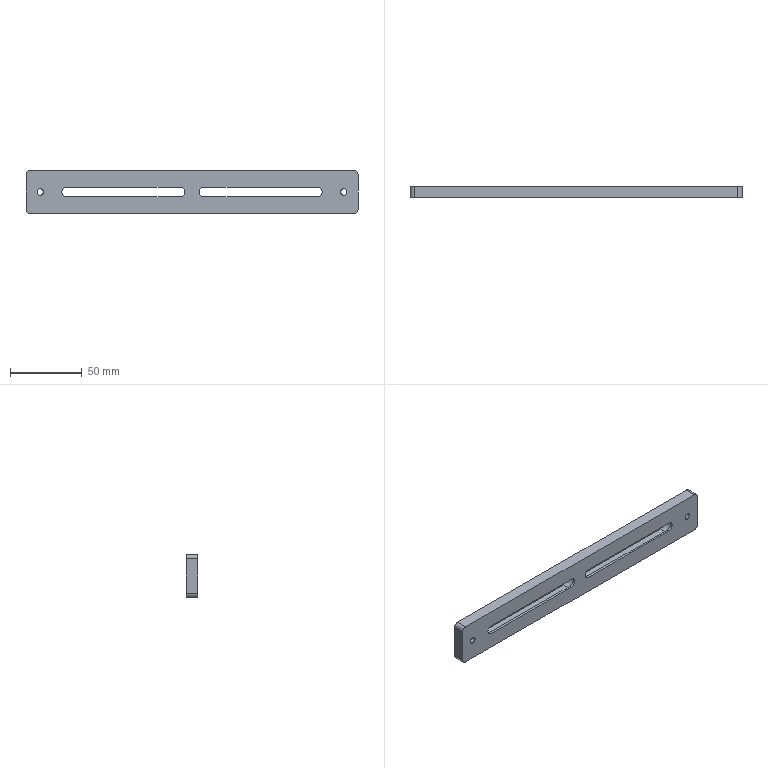Part | SolidWorks | features BaseBody 1 | 1 solid | 38 faces | box 232 x 8 x 30 mm | volume 40879 mm3 | cylinder 20 | plane 18 | commonest cylinder face diameters 4.5 x4 6 x4 6.6 x4 8 x4 11 x4
STEP:
#1=CARTESIAN_POINT('',(-106.,0.,-2.25));
#2=VERTEX_POINT('',#1);
#3=CARTESIAN_POINT('',(-106.,0.,2.25));
#4=VERTEX_POINT('',#3);
#5=CARTESIAN_POINT('',(-106.,0.,0.));
#6=DIRECTION('',(0.,1.,0.));
#7=DIRECTION('',(0.,0.,1.));
#8=AXIS2_PLACEMENT_3D('',#5,#6,#7);
#9=CIRCLE('',#8,2.25);
#10=EDGE_CURVE('',#2,#4,#9,.T.);
#11=ORIENTED_EDGE('',*,*,#10,.F.);
#12=CARTESIAN_POINT('',(-106.,3.6,-2.25));
#13=VERTEX_POINT('',#12);
#14=CARTESIAN_POINT('',(-106.,8.,-2.25));
#15=DIRECTION('',(0.,1.,0.));
#16=VECTOR('',#15,1000.);
#17=LINE('',#14,#16);
#18=EDGE_CURVE('',#2,#13,#17,.T.);
#19=ORIENTED_EDGE('',*,*,#18,.T.);
#20=CARTESIAN_POINT('',(-106.,3.6,2.25));
#21=VERTEX_POINT('',#20);
#22=CARTESIAN_POINT('',(-106.,3.6,0.));
#23=DIRECTION('',(0.,-1.,0.));
#24=DIRECTION('',(0.,0.,1.));
#25=AXIS2_PLACEMENT_3D('',#22,#23,#24);
#26=CIRCLE('',#25,2.25);
#27=EDGE_CURVE('',#21,#13,#26,.T.);
#28=ORIENTED_EDGE('',*,*,#27,.F.);
#29=CARTESIAN_POINT('',(-106.,8.,2.25));
#30=DIRECTION('',(0.,1.,0.));
#31=VECTOR('',#30,1000.);
#32=LINE('',#29,#31);
#33=EDGE_CURVE('',#4,#21,#32,.T.);
#34=ORIENTED_EDGE('',*,*,#33,.F.);
#35=EDGE_LOOP('',(#11,#19,#28,#34));
#36=FACE_OUTER_BOUND('',#35,.T.);
#37=CARTESIAN_POINT('',(-106.,8.,0.));
#38=DIRECTION('',(0.,1.,0.));
#39=DIRECTION('',(0.,0.,1.));
#40=AXIS2_PLACEMENT_3D('',#37,#38,#39);
#41=CYLINDRICAL_SURFACE('',#40,2.25);
#42=ADVANCED_FACE('',(#36),#41,.F.);
#43=CARTESIAN_POINT('',(106.,0.,-2.25));
#44=VERTEX_POINT('',#43);
#45=CARTESIAN_POINT('',(106.,0.,2.25));
#46=VERTEX_POINT('',#45);
#47=CARTESIAN_POINT('',(106.,0.,0.));
#48=DIRECTION('',(0.,1.,0.));
#49=DIRECTION('',(0.,0.,1.));
#50=AXIS2_PLACEMENT_3D('',#47,#48,#49);
#51=CIRCLE('',#50,2.25);
#52=EDGE_CURVE('',#44,#46,#51,.T.);
#53=ORIENTED_EDGE('',*,*,#52,.F.);
#54=CARTESIAN_POINT('',(106.,3.6,-2.25));
#55=VERTEX_POINT('',#54);
#56=CARTESIAN_POINT('',(106.,8.,-2.25));
#57=DIRECTION('',(0.,1.,0.));
#58=VECTOR('',#57,1000.);
#59=LINE('',#56,#58);
#60=EDGE_CURVE('',#44,#55,#59,.T.);
#61=ORIENTED_EDGE('',*,*,#60,.T.);
#62=CARTESIAN_POINT('',(106.,3.6,2.25));
#63=VERTEX_POINT('',#62);
#64=CARTESIAN_POINT('',(106.,3.6,0.));
#65=DIRECTION('',(0.,-1.,0.));
#66=DIRECTION('',(0.,0.,1.));
#67=AXIS2_PLACEMENT_3D('',#64,#65,#66);
#68=CIRCLE('',#67,2.25);
#69=EDGE_CURVE('',#63,#55,#68,.T.);
#70=ORIENTED_EDGE('',*,*,#69,.F.);
#71=CARTESIAN_POINT('',(106.,8.,2.25));
#72=DIRECTION('',(0.,1.,0.));
#73=VECTOR('',#72,1000.);
#74=LINE('',#71,#73);
#75=EDGE_CURVE('',#46,#63,#74,.T.);
#76=ORIENTED_EDGE('',*,*,#75,.F.);
#77=EDGE_LOOP('',(#53,#61,#70,#76));
#78=FACE_OUTER_BOUND('',#77,.T.);
#79=CARTESIAN_POINT('',(106.,8.,0.));
#80=DIRECTION('',(0.,1.,0.));
#81=DIRECTION('',(0.,0.,1.));
#82=AXIS2_PLACEMENT_3D('',#79,#80,#81);
#83=CYLINDRICAL_SURFACE('',#82,2.25);
#84=ADVANCED_FACE('',(#78),#83,.F.);
#85=CARTESIAN_POINT('',(-106.,3.6,4.));
#86=VERTEX_POINT('',#85);
#87=CARTESIAN_POINT('',(-106.,3.6,-4.));
#88=VERTEX_POINT('',#87);
#89=CARTESIAN_POINT('',(-106.,3.6,0.));
#90=DIRECTION('',(0.,-1.,0.));
#91=DIRECTION('',(0.,0.,1.));
#92=AXIS2_PLACEMENT_3D('',#89,#90,#91);
#93=CIRCLE('',#92,4.);
#94=EDGE_CURVE('',#86,#88,#93,.T.);
#95=ORIENTED_EDGE('',*,*,#94,.T.);
#96=CARTESIAN_POINT('',(-106.,8.,-4.));
#97=VERTEX_POINT('',#96);
#98=CARTESIAN_POINT('',(-106.,8.,-4.));
#99=DIRECTION('',(0.,1.,0.));
#100=VECTOR('',#99,1000.);
#101=LINE('',#98,#100);
#102=EDGE_CURVE('',#88,#97,#101,.T.);
#103=ORIENTED_EDGE('',*,*,#102,.T.);
#104=CARTESIAN_POINT('',(-106.,8.,4.));
#105=VERTEX_POINT('',#104);
#106=CARTESIAN_POINT('',(-106.,8.,0.));
#107=DIRECTION('',(0.,1.,0.));
#108=DIRECTION('',(0.,0.,1.));
#109=AXIS2_PLACEMENT_3D('',#106,#107,#108);
#110=CIRCLE('',#109,4.);
#111=EDGE_CURVE('',#97,#105,#110,.T.);
#112=ORIENTED_EDGE('',*,*,#111,.T.);
#113=CARTESIAN_POINT('',(-106.,8.,4.));
#114=DIRECTION('',(0.,1.,0.));
#115=VECTOR('',#114,1000.);
#116=LINE('',#113,#115);
#117=EDGE_CURVE('',#86,#105,#116,.T.);
#118=ORIENTED_EDGE('',*,*,#117,.F.);
#119=EDGE_LOOP('',(#95,#103,#112,#118));
#120=FACE_OUTER_BOUND('',#119,.T.);
#121=CARTESIAN_POINT('',(-106.,8.,0.));
#122=DIRECTION('',(0.,1.,0.));
#123=DIRECTION('',(0.,0.,1.));
#124=AXIS2_PLACEMENT_3D('',#121,#122,#123);
#125=CYLINDRICAL_SURFACE('',#124,4.);
#126=ADVANCED_FACE('',(#120),#125,.F.);
#127=CARTESIAN_POINT('',(106.,3.6,4.));
#128=VERTEX_POINT('',#127);
#129=CARTESIAN_POINT('',(106.,3.6,-4.));
#130=VERTEX_POINT('',#129);
#131=CARTESIAN_POINT('',(106.,3.6,0.));
#132=DIRECTION('',(0.,-1.,0.));
#133=DIRECTION('',(0.,0.,1.));
#134=AXIS2_PLACEMENT_3D('',#131,#132,#133);
#135=CIRCLE('',#134,4.);
#136=EDGE_CURVE('',#128,#130,#135,.T.);
#137=ORIENTED_EDGE('',*,*,#136,.T.);
#138=CARTESIAN_POINT('',(106.,8.,-4.));
#139=VERTEX_POINT('',#138);
#140=CARTESIAN_POINT('',(106.,8.,-4.));
#141=DIRECTION('',(0.,1.,0.));
#142=VECTOR('',#141,1000.);
#143=LINE('',#140,#142);
#144=EDGE_CURVE('',#130,#139,#143,.T.);
#145=ORIENTED_EDGE('',*,*,#144,.T.);
#146=CARTESIAN_POINT('',(106.,8.,4.));
#147=VERTEX_POINT('',#146);
#148=CARTESIAN_POINT('',(106.,8.,0.));
#149=DIRECTION('',(0.,1.,0.));
#150=DIRECTION('',(0.,0.,1.));
#151=AXIS2_PLACEMENT_3D('',#148,#149,#150);
#152=CIRCLE('',#151,4.);
#153=EDGE_CURVE('',#139,#147,#152,.T.);
#154=ORIENTED_EDGE('',*,*,#153,.T.);
#155=CARTESIAN_POINT('',(106.,8.,4.));
#156=DIRECTION('',(0.,1.,0.));
#157=VECTOR('',#156,1000.);
#158=LINE('',#155,#157);
#159=EDGE_CURVE('',#128,#147,#158,.T.);
#160=ORIENTED_EDGE('',*,*,#159,.F.);
#161=EDGE_LOOP('',(#137,#145,#154,#160));
#162=FACE_OUTER_BOUND('',#161,.T.);
#163=CARTESIAN_POINT('',(106.,8.,0.));
#164=DIRECTION('',(0.,1.,0.));
#165=DIRECTION('',(0.,0.,1.));
#166=AXIS2_PLACEMENT_3D('',#163,#164,#165);
#167=CYLINDRICAL_SURFACE('',#166,4.);
#168=ADVANCED_FACE('',(#162),#167,.F.);
#169=CARTESIAN_POINT('',(87.7,1.6,5.5));
#170=VERTEX_POINT('',#169);
#171=CARTESIAN_POINT('',(8.3,1.6,5.5));
#172=VERTEX_POINT('',#171);
#173=CARTESIAN_POINT('',(91.,1.6,5.5));
#174=DIRECTION('',(-1.,0.,0.));
#175=VECTOR('',#174,1000.);
#176=LINE('',#173,#175);
#177=EDGE_CURVE('',#170,#172,#176,.T.);
#178=ORIENTED_EDGE('',*,*,#177,.T.);
#179=CARTESIAN_POINT('',(8.3,8.,5.5));
#180=VERTEX_POINT('',#179);
#181=CARTESIAN_POINT('',(8.3,8.,5.5));
#182=DIRECTION('',(0.,1.,0.));
#183=VECTOR('',#182,1000.);
#184=LINE('',#181,#183);
#185=EDGE_CURVE('',#172,#180,#184,.T.);
#186=ORIENTED_EDGE('',*,*,#185,.T.);
#187=CARTESIAN_POINT('',(87.7,8.,5.5));
#188=VERTEX_POINT('',#187);
#189=CARTESIAN_POINT('',(0.,8.,5.5));
#190=DIRECTION('',(1.,0.,0.));
#191=VECTOR('',#190,1000.);
#192=LINE('',#189,#191);
#193=EDGE_CURVE('',#180,#188,#192,.T.);
#194=ORIENTED_EDGE('',*,*,#193,.T.);
#195=CARTESIAN_POINT('',(87.7,8.,5.5));
#196=DIRECTION('',(0.,-1.,0.));
#197=VECTOR('',#196,1000.);
#198=LINE('',#195,#197);
#199=EDGE_CURVE('',#188,#170,#198,.T.);
#200=ORIENTED_EDGE('',*,*,#199,.T.);
#201=EDGE_LOOP('',(#178,#186,#194,#200));
#202=FACE_OUTER_BOUND('',#201,.T.);
#203=CARTESIAN_POINT('',(8.3,8.,5.5));
#204=DIRECTION('',(0.,0.,1.));
#205=DIRECTION('',(1.,0.,0.));
#206=AXIS2_PLACEMENT_3D('',#203,#204,#205);
#207=PLANE('',#206);
#208=ADVANCED_FACE('',(#202),#207,.F.);
#209=ORIENTED_EDGE('',*,*,#185,.F.);
#210=CARTESIAN_POINT('',(8.3,1.6,-5.5));
#211=VERTEX_POINT('',#210);
#212=CARTESIAN_POINT('',(8.3,1.6,0.));
#213=DIRECTION('',(0.,-1.,0.));
#214=DIRECTION('',(0.,0.,1.));
#215=AXIS2_PLACEMENT_3D('',#212,#213,#214);
#216=CIRCLE('',#215,5.5);
#217=EDGE_CURVE('',#172,#211,#216,.T.);
#218=ORIENTED_EDGE('',*,*,#217,.T.);
#219=CARTESIAN_POINT('',(8.3,8.,-5.5));
#220=VERTEX_POINT('',#219);
#221=CARTESIAN_POINT('',(8.3,8.,-5.5));
#222=DIRECTION('',(0.,1.,0.));
#223=VECTOR('',#222,1000.);
#224=LINE('',#221,#223);
#225=EDGE_CURVE('',#211,#220,#224,.T.);
#226=ORIENTED_EDGE('',*,*,#225,.T.);
#227=CARTESIAN_POINT('',(8.3,8.,0.));
#228=DIRECTION('',(0.,1.,0.));
#229=DIRECTION('',(0.,0.,1.));
#230=AXIS2_PLACEMENT_3D('',#227,#228,#229);
#231=CIRCLE('',#230,5.5);
#232=EDGE_CURVE('',#220,#180,#231,.T.);
#233=ORIENTED_EDGE('',*,*,#232,.T.);
#234=EDGE_LOOP('',(#209,#218,#226,#233));
#235=FACE_OUTER_BOUND('',#234,.T.);
#236=CARTESIAN_POINT('',(8.3,8.,0.));
#237=DIRECTION('',(0.,1.,0.));
#238=DIRECTION('',(0.,0.,1.));
#239=AXIS2_PLACEMENT_3D('',#236,#237,#238);
#240=CYLINDRICAL_SURFACE('',#239,5.5);
#241=ADVANCED_FACE('',(#235),#240,.F.);
#242=CARTESIAN_POINT('',(87.7,8.,-5.5));
#243=VERTEX_POINT('',#242);
#244=CARTESIAN_POINT('',(0.,8.,-5.5));
#245=DIRECTION('',(-1.,0.,0.));
#246=VECTOR('',#245,1000.);
#247=LINE('',#244,#246);
#248=EDGE_CURVE('',#243,#220,#247,.T.);
#249=ORIENTED_EDGE('',*,*,#248,.T.);
#250=ORIENTED_EDGE('',*,*,#225,.F.);
#251=CARTESIAN_POINT('',(87.7,1.6,-5.5));
#252=VERTEX_POINT('',#251);
#253=CARTESIAN_POINT('',(91.,1.6,-5.5));
#254=DIRECTION('',(1.,0.,0.));
#255=VECTOR('',#254,1000.);
#256=LINE('',#253,#255);
#257=EDGE_CURVE('',#211,#252,#256,.T.);
#258=ORIENTED_EDGE('',*,*,#257,.T.);
#259=CARTESIAN_POINT('',(87.7,8.,-5.5));
#260=DIRECTION('',(0.,1.,0.));
#261=VECTOR('',#260,1000.);
#262=LINE('',#259,#261);
#263=EDGE_CURVE('',#252,#243,#262,.T.);
#264=ORIENTED_EDGE('',*,*,#263,.T.);
#265=EDGE_LOOP('',(#249,#250,#258,#264));
#266=FACE_OUTER_BOUND('',#265,.T.);
#267=CARTESIAN_POINT('',(8.3,8.,-5.5));
#268=DIRECTION('',(0.,0.,-1.));
#269=DIRECTION('',(-1.,0.,0.));
#270=AXIS2_PLACEMENT_3D('',#267,#268,#269);
#271=PLANE('',#270);
#272=ADVANCED_FACE('',(#266),#271,.F.);
#273=ORIENTED_EDGE('',*,*,#199,.F.);
#274=CARTESIAN_POINT('',(87.7,8.,0.));
#275=DIRECTION('',(0.,1.,0.));
#276=DIRECTION('',(0.,0.,1.));
#277=AXIS2_PLACEMENT_3D('',#274,#275,#276);
#278=CIRCLE('',#277,5.5);
#279=EDGE_CURVE('',#188,#243,#278,.T.);
#280=ORIENTED_EDGE('',*,*,#279,.T.);
#281=ORIENTED_EDGE('',*,*,#263,.F.);
#282=CARTESIAN_POINT('',(87.7,1.6,0.));
#283=DIRECTION('',(0.,-1.,0.));
#284=DIRECTION('',(0.,0.,1.));
#285=AXIS2_PLACEMENT_3D('',#282,#283,#284);
#286=CIRCLE('',#285,5.5);
#287=EDGE_CURVE('',#252,#170,#286,.T.);
#288=ORIENTED_EDGE('',*,*,#287,.T.);
#289=EDGE_LOOP('',(#273,#280,#281,#288));
#290=FACE_OUTER_BOUND('',#289,.T.);
#291=CARTESIAN_POINT('',(87.7,8.,0.));
#292=DIRECTION('',(0.,1.,0.));
#293=DIRECTION('',(0.,0.,1.));
#294=AXIS2_PLACEMENT_3D('',#291,#292,#293);
#295=CYLINDRICAL_SURFACE('',#294,5.5);
#296=ADVANCED_FACE('',(#290),#295,.F.);
#297=CARTESIAN_POINT('',(-8.3,1.6,5.5));
#298=VERTEX_POINT('',#297);
#299=CARTESIAN_POINT('',(-87.7,1.6,5.5));
#300=VERTEX_POINT('',#299);
#301=CARTESIAN_POINT('',(-5.,1.6,5.5));
#302=DIRECTION('',(-1.,0.,0.));
#303=VECTOR('',#302,1000.);
#304=LINE('',#301,#303);
#305=EDGE_CURVE('',#298,#300,#304,.T.);
#306=ORIENTED_EDGE('',*,*,#305,.T.);
#307=CARTESIAN_POINT('',(-87.7,8.,5.5));
#308=VERTEX_POINT('',#307);
#309=CARTESIAN_POINT('',(-87.7,8.,5.5));
#310=DIRECTION('',(0.,1.,0.));
#311=VECTOR('',#310,1000.);
#312=LINE('',#309,#311);
#313=EDGE_CURVE('',#300,#308,#312,.T.);
#314=ORIENTED_EDGE('',*,*,#313,.T.);
#315=CARTESIAN_POINT('',(-8.3,8.,5.5));
#316=VERTEX_POINT('',#315);
#317=CARTESIAN_POINT('',(0.,8.,5.5));
#318=DIRECTION('',(1.,0.,0.));
#319=VECTOR('',#318,1000.);
#320=LINE('',#317,#319);
#321=EDGE_CURVE('',#308,#316,#320,.T.);
#322=ORIENTED_EDGE('',*,*,#321,.T.);
#323=CARTESIAN_POINT('',(-8.3,8.,5.5));
#324=DIRECTION('',(0.,-1.,0.));
#325=VECTOR('',#324,1000.);
#326=LINE('',#323,#325);
#327=EDGE_CURVE('',#316,#298,#326,.T.);
#328=ORIENTED_EDGE('',*,*,#327,.T.);
#329=EDGE_LOOP('',(#306,#314,#322,#328));
#330=FACE_OUTER_BOUND('',#329,.T.);
#331=CARTESIAN_POINT('',(-87.7,8.,5.5));
#332=DIRECTION('',(0.,0.,1.));
#333=DIRECTION('',(1.,0.,0.));
#334=AXIS2_PLACEMENT_3D('',#331,#332,#333);
#335=PLANE('',#334);
#336=ADVANCED_FACE('',(#330),#335,.F.);
#337=ORIENTED_EDGE('',*,*,#313,.F.);
#338=CARTESIAN_POINT('',(-87.7,1.6,-5.5));
#339=VERTEX_POINT('',#338);
#340=CARTESIAN_POINT('',(-87.7,1.6,0.));
#341=DIRECTION('',(0.,-1.,0.));
#342=DIRECTION('',(0.,0.,1.));
#343=AXIS2_PLACEMENT_3D('',#340,#341,#342);
#344=CIRCLE('',#343,5.5);
#345=EDGE_CURVE('',#300,#339,#344,.T.);
#346=ORIENTED_EDGE('',*,*,#345,.T.);
#347=CARTESIAN_POINT('',(-87.7,8.,-5.5));
#348=VERTEX_POINT('',#347);
#349=CARTESIAN_POINT('',(-87.7,8.,-5.5));
#350=DIRECTION('',(0.,1.,0.));
#351=VECTOR('',#350,1000.);
#352=LINE('',#349,#351);
#353=EDGE_CURVE('',#339,#348,#352,.T.);
#354=ORIENTED_EDGE('',*,*,#353,.T.);
#355=CARTESIAN_POINT('',(-87.7,8.,0.));
#356=DIRECTION('',(0.,1.,0.));
#357=DIRECTION('',(0.,0.,1.));
#358=AXIS2_PLACEMENT_3D('',#355,#356,#357);
#359=CIRCLE('',#358,5.5);
#360=EDGE_CURVE('',#348,#308,#359,.T.);
#361=ORIENTED_EDGE('',*,*,#360,.T.);
#362=EDGE_LOOP('',(#337,#346,#354,#361));
#363=FACE_OUTER_BOUND('',#362,.T.);
#364=CARTESIAN_POINT('',(-87.7,8.,0.));
#365=DIRECTION('',(0.,1.,0.));
#366=DIRECTION('',(0.,0.,1.));
#367=AXIS2_PLACEMENT_3D('',#364,#365,#366);
#368=CYLINDRICAL_SURFACE('',#367,5.5);
#369=ADVANCED_FACE('',(#363),#368,.F.);
#370=CARTESIAN_POINT('',(-8.3,8.,-5.5));
#371=VERTEX_POINT('',#370);
#372=CARTESIAN_POINT('',(0.,8.,-5.5));
#373=DIRECTION('',(-1.,0.,0.));
#374=VECTOR('',#373,1000.);
#375=LINE('',#372,#374);
#376=EDGE_CURVE('',#371,#348,#375,.T.);
#377=ORIENTED_EDGE('',*,*,#376,.T.);
#378=ORIENTED_EDGE('',*,*,#353,.F.);
#379=CARTESIAN_POINT('',(-8.3,1.6,-5.5));
#380=VERTEX_POINT('',#379);
#381=CARTESIAN_POINT('',(-5.,1.6,-5.5));
#382=DIRECTION('',(1.,0.,0.));
#383=VECTOR('',#382,1000.);
#384=LINE('',#381,#383);
#385=EDGE_CURVE('',#339,#380,#384,.T.);
#386=ORIENTED_EDGE('',*,*,#385,.T.);
#387=CARTESIAN_POINT('',(-8.3,8.,-5.5));
#388=DIRECTION('',(0.,1.,0.));
#389=VECTOR('',#388,1000.);
#390=LINE('',#387,#389);
#391=EDGE_CURVE('',#380,#371,#390,.T.);
#392=ORIENTED_EDGE('',*,*,#391,.T.);
#393=EDGE_LOOP('',(#377,#378,#386,#392));
#394=FACE_OUTER_BOUND('',#393,.T.);
#395=CARTESIAN_POINT('',(-87.7,8.,-5.5));
#396=DIRECTION('',(0.,0.,-1.));
#397=DIRECTION('',(-1.,0.,0.));
#398=AXIS2_PLACEMENT_3D('',#395,#396,#397);
#399=PLANE('',#398);
#400=ADVANCED_FACE('',(#394),#399,.F.);
#401=ORIENTED_EDGE('',*,*,#327,.F.);
#402=CARTESIAN_POINT('',(-8.3,8.,0.));
#403=DIRECTION('',(0.,1.,0.));
#404=DIRECTION('',(0.,0.,1.));
#405=AXIS2_PLACEMENT_3D('',#402,#403,#404);
#406=CIRCLE('',#405,5.5);
#407=EDGE_CURVE('',#316,#371,#406,.T.);
#408=ORIENTED_EDGE('',*,*,#407,.T.);
#409=ORIENTED_EDGE('',*,*,#391,.F.);
#410=CARTESIAN_POINT('',(-8.3,1.6,0.));
#411=DIRECTION('',(0.,-1.,0.));
#412=DIRECTION('',(0.,0.,1.));
#413=AXIS2_PLACEMENT_3D('',#410,#411,#412);
#414=CIRCLE('',#413,5.5);
#415=EDGE_CURVE('',#380,#298,#414,.T.);
#416=ORIENTED_EDGE('',*,*,#415,.T.);
#417=EDGE_LOOP('',(#401,#408,#409,#416));
#418=FACE_OUTER_BOUND('',#417,.T.);
#419=CARTESIAN_POINT('',(-8.3,8.,0.));
#420=DIRECTION('',(0.,1.,0.));
#421=DIRECTION('',(0.,0.,1.));
#422=AXIS2_PLACEMENT_3D('',#419,#420,#421);
#423=CYLINDRICAL_SURFACE('',#422,5.5);
#424=ADVANCED_FACE('',(#418),#423,.F.);
#425=ORIENTED_EDGE('',*,*,#360,.F.);
#426=ORIENTED_EDGE('',*,*,#376,.F.);
#427=ORIENTED_EDGE('',*,*,#407,.F.);
#428=ORIENTED_EDGE('',*,*,#321,.F.);
#429=EDGE_LOOP('',(#425,#426,#427,#428));
#430=FACE_BOUND('',#429,.T.);
#431=ORIENTED_EDGE('',*,*,#248,.F.);
#432=ORIENTED_EDGE('',*,*,#279,.F.);
#433=ORIENTED_EDGE('',*,*,#193,.F.);
#434=ORIENTED_EDGE('',*,*,#232,.F.);
#435=EDGE_LOOP('',(#431,#432,#433,#434));
#436=FACE_BOUND('',#435,.T.);
#437=CARTESIAN_POINT('',(-106.,8.,0.));
#438=DIRECTION('',(0.,1.,0.));
#439=DIRECTION('',(0.,0.,1.));
#440=AXIS2_PLACEMENT_3D('',#437,#438,#439);
#441=CIRCLE('',#440,4.);
#442=EDGE_CURVE('',#105,#97,#441,.T.);
#443=ORIENTED_EDGE('',*,*,#442,.F.);
#444=ORIENTED_EDGE('',*,*,#111,.F.);
#445=EDGE_LOOP('',(#443,#444));
#446=FACE_BOUND('',#445,.T.);
#447=CARTESIAN_POINT('',(106.,8.,0.));
#448=DIRECTION('',(0.,1.,0.));
#449=DIRECTION('',(0.,0.,1.));
#450=AXIS2_PLACEMENT_3D('',#447,#448,#449);
#451=CIRCLE('',#450,4.);
#452=EDGE_CURVE('',#147,#139,#451,.T.);
#453=ORIENTED_EDGE('',*,*,#452,.F.);
#454=ORIENTED_EDGE('',*,*,#153,.F.);
#455=EDGE_LOOP('',(#453,#454));
#456=FACE_BOUND('',#455,.T.);
#457=CARTESIAN_POINT('',(-113.,8.,15.));
#458=VERTEX_POINT('',#457);
#459=CARTESIAN_POINT('',(-116.,8.,12.));
#460=VERTEX_POINT('',#459);
#461=CARTESIAN_POINT('',(-113.,8.,12.));
#462=DIRECTION('',(0.,-1.,0.));
#463=DIRECTION('',(0.,0.,-1.));
#464=AXIS2_PLACEMENT_3D('',#461,#462,#463);
#465=CIRCLE('',#464,3.);
#466=EDGE_CURVE('',#458,#460,#465,.T.);
#467=ORIENTED_EDGE('',*,*,#466,.F.);
#468=CARTESIAN_POINT('',(113.,8.,15.));
#469=VERTEX_POINT('',#468);
#470=CARTESIAN_POINT('',(-116.,8.,15.));
#471=DIRECTION('',(1.,0.,0.));
#472=VECTOR('',#471,1000.);
#473=LINE('',#470,#472);
#474=EDGE_CURVE('',#458,#469,#473,.T.);
#475=ORIENTED_EDGE('',*,*,#474,.T.);
#476=CARTESIAN_POINT('',(116.,8.,12.));
#477=VERTEX_POINT('',#476);
#478=CARTESIAN_POINT('',(113.,8.,12.));
#479=DIRECTION('',(0.,-1.,0.));
#480=DIRECTION('',(0.,0.,-1.));
#481=AXIS2_PLACEMENT_3D('',#478,#479,#480);
#482=CIRCLE('',#481,3.);
#483=EDGE_CURVE('',#477,#469,#482,.T.);
#484=ORIENTED_EDGE('',*,*,#483,.F.);
#485=CARTESIAN_POINT('',(116.,8.,-12.));
#486=VERTEX_POINT('',#485);
#487=CARTESIAN_POINT('',(116.,8.,15.));
#488=DIRECTION('',(0.,0.,-1.));
#489=VECTOR('',#488,1000.);
#490=LINE('',#487,#489);
#491=EDGE_CURVE('',#477,#486,#490,.T.);
#492=ORIENTED_EDGE('',*,*,#491,.T.);
#493=CARTESIAN_POINT('',(113.,8.,-15.));
#494=VERTEX_POINT('',#493);
#495=CARTESIAN_POINT('',(113.,8.,-12.));
#496=DIRECTION('',(0.,-1.,0.));
#497=DIRECTION('',(0.,0.,-1.));
#498=AXIS2_PLACEMENT_3D('',#495,#496,#497);
#499=CIRCLE('',#498,3.);
#500=EDGE_CURVE('',#494,#486,#499,.T.);
#501=ORIENTED_EDGE('',*,*,#500,.F.);
#502=CARTESIAN_POINT('',(-113.,8.,-15.));
#503=VERTEX_POINT('',#502);
#504=CARTESIAN_POINT('',(-116.,8.,-15.));
#505=DIRECTION('',(-1.,0.,0.));
#506=VECTOR('',#505,1000.);
#507=LINE('',#504,#506);
#508=EDGE_CURVE('',#494,#503,#507,.T.);
#509=ORIENTED_EDGE('',*,*,#508,.T.);
#510=CARTESIAN_POINT('',(-116.,8.,-12.));
#511=VERTEX_POINT('',#510);
#512=CARTESIAN_POINT('',(-113.,8.,-12.));
#513=DIRECTION('',(0.,-1.,0.));
#514=DIRECTION('',(0.,0.,-1.));
#515=AXIS2_PLACEMENT_3D('',#512,#513,#514);
#516=CIRCLE('',#515,3.);
#517=EDGE_CURVE('',#511,#503,#516,.T.);
#518=ORIENTED_EDGE('',*,*,#517,.F.);
#519=CARTESIAN_POINT('',(-116.,8.,15.));
#520=DIRECTION('',(0.,0.,1.));
#521=VECTOR('',#520,1000.);
#522=LINE('',#519,#521);
#523=EDGE_CURVE('',#511,#460,#522,.T.);
#524=ORIENTED_EDGE('',*,*,#523,.T.);
#525=EDGE_LOOP('',(#467,#475,#484,#492,#501,#509,#518,#524));
#526=FACE_OUTER_BOUND('',#525,.T.);
#527=CARTESIAN_POINT('',(0.,8.,0.));
#528=DIRECTION('',(0.,-1.,0.));
#529=DIRECTION('',(0.,0.,-1.));
#530=AXIS2_PLACEMENT_3D('',#527,#528,#529);
#531=PLANE('',#530);
#532=ADVANCED_FACE('',(#430,#436,#446,#456,#526),#531,.F.);
#533=ORIENTED_EDGE('',*,*,#69,.T.);
#534=CARTESIAN_POINT('',(106.,3.6,0.));
#535=DIRECTION('',(0.,-1.,0.));
#536=DIRECTION('',(0.,0.,1.));
#537=AXIS2_PLACEMENT_3D('',#534,#535,#536);
#538=CIRCLE('',#537,2.25);
#539=EDGE_CURVE('',#55,#63,#538,.T.);
#540=ORIENTED_EDGE('',*,*,#539,.T.);
#541=EDGE_LOOP('',(#533,#540));
#542=FACE_BOUND('',#541,.T.);
#543=ORIENTED_EDGE('',*,*,#136,.F.);
#544=CARTESIAN_POINT('',(106.,3.6,0.));
#545=DIRECTION('',(0.,-1.,0.));
#546=DIRECTION('',(0.,0.,1.));
#547=AXIS2_PLACEMENT_3D('',#544,#545,#546);
#548=CIRCLE('',#547,4.);
#549=EDGE_CURVE('',#130,#128,#548,.T.);
#550=ORIENTED_EDGE('',*,*,#549,.F.);
#551=EDGE_LOOP('',(#543,#550));
#552=FACE_OUTER_BOUND('',#551,.T.);
#553=CARTESIAN_POINT('',(108.25,3.6,0.));
#554=DIRECTION('',(0.,-1.,0.));
#555=DIRECTION('',(0.,0.,-1.));
#556=AXIS2_PLACEMENT_3D('',#553,#554,#555);
#557=PLANE('',#556);
#558=ADVANCED_FACE('',(#542,#552),#557,.F.);
#559=ORIENTED_EDGE('',*,*,#27,.T.);
#560=CARTESIAN_POINT('',(-106.,3.6,0.));
#561=DIRECTION('',(0.,-1.,0.));
#562=DIRECTION('',(0.,0.,1.));
#563=AXIS2_PLACEMENT_3D('',#560,#561,#562);
#564=CIRCLE('',#563,2.25);
#565=EDGE_CURVE('',#13,#21,#564,.T.);
#566=ORIENTED_EDGE('',*,*,#565,.T.);
#567=EDGE_LOOP('',(#559,#566));
#568=FACE_BOUND('',#567,.T.);
#569=ORIENTED_EDGE('',*,*,#94,.F.);
#570=CARTESIAN_POINT('',(-106.,3.6,0.));
#571=DIRECTION('',(0.,-1.,0.));
#572=DIRECTION('',(0.,0.,1.));
#573=AXIS2_PLACEMENT_3D('',#570,#571,#572);
#574=CIRCLE('',#573,4.);
#575=EDGE_CURVE('',#88,#86,#574,.T.);
#576=ORIENTED_EDGE('',*,*,#575,.F.);
#577=EDGE_LOOP('',(#569,#576));
#578=FACE_OUTER_BOUND('',#577,.T.);
#579=CARTESIAN_POINT('',(-103.75,3.6,0.));
#580=DIRECTION('',(0.,-1.,0.));
#581=DIRECTION('',(0.,0.,-1.));
#582=AXIS2_PLACEMENT_3D('',#579,#580,#581);
#583=PLANE('',#582);
#584=ADVANCED_FACE('',(#568,#578),#583,.F.);
#585=CARTESIAN_POINT('',(8.3,1.6,3.3));
#586=VERTEX_POINT('',#585);
#587=CARTESIAN_POINT('',(8.3,1.6,-3.3));
#588=VERTEX_POINT('',#587);
#589=CARTESIAN_POINT('',(8.3,1.6,0.));
#590=DIRECTION('',(0.,-1.,0.));
#591=DIRECTION('',(0.,0.,1.));
#592=AXIS2_PLACEMENT_3D('',#589,#590,#591);
#593=CIRCLE('',#592,3.3);
#594=EDGE_CURVE('',#586,#588,#593,.T.);
#595=ORIENTED_EDGE('',*,*,#594,.T.);
#596=CARTESIAN_POINT('',(87.7,1.6,-3.3));
#597=VERTEX_POINT('',#596);
#598=CARTESIAN_POINT('',(8.3,1.6,-3.3));
#599=DIRECTION('',(1.,0.,0.));
#600=VECTOR('',#599,1000.);
#601=LINE('',#598,#600);
#602=EDGE_CURVE('',#588,#597,#601,.T.);
#603=ORIENTED_EDGE('',*,*,#602,.T.);
#604=CARTESIAN_POINT('',(87.7,1.6,3.3));
#605=VERTEX_POINT('',#604);
#606=CARTESIAN_POINT('',(87.7,1.6,0.));
#607=DIRECTION('',(0.,-1.,0.));
#608=DIRECTION('',(0.,0.,1.));
#609=AXIS2_PLACEMENT_3D('',#606,#607,#608);
#610=CIRCLE('',#609,3.3);
#611=EDGE_CURVE('',#597,#605,#610,.T.);
#612=ORIENTED_EDGE('',*,*,#611,.T.);
#613=CARTESIAN_POINT('',(8.3,1.6,3.3));
#614=DIRECTION('',(-1.,0.,0.));
#615=VECTOR('',#614,1000.);
#616=LINE('',#613,#615);
#617=EDGE_CURVE('',#605,#586,#616,.T.);
#618=ORIENTED_EDGE('',*,*,#617,.T.);
#619=EDGE_LOOP('',(#595,#603,#612,#618));
#620=FACE_BOUND('',#619,.T.);
#621=ORIENTED_EDGE('',*,*,#257,.F.);
#622=ORIENTED_EDGE('',*,*,#217,.F.);
#623=ORIENTED_EDGE('',*,*,#177,.F.);
#624=ORIENTED_EDGE('',*,*,#287,.F.);
#625=EDGE_LOOP('',(#621,#622,#623,#624));
#626=FACE_OUTER_BOUND('',#625,.T.);
#627=CARTESIAN_POINT('',(91.,1.6,0.));
#628=DIRECTION('',(0.,-1.,0.));
#629=DIRECTION('',(0.,0.,-1.));
#630=AXIS2_PLACEMENT_3D('',#627,#628,#629);
#631=PLANE('',#630);
#632=ADVANCED_FACE('',(#620,#626),#631,.F.);
#633=CARTESIAN_POINT('',(-87.7,1.6,3.3));
#634=VERTEX_POINT('',#633);
#635=CARTESIAN_POINT('',(-87.7,1.6,-3.3));
#636=VERTEX_POINT('',#635);
#637=CARTESIAN_POINT('',(-87.7,1.6,0.));
#638=DIRECTION('',(0.,-1.,0.));
#639=DIRECTION('',(0.,0.,1.));
#640=AXIS2_PLACEMENT_3D('',#637,#638,#639);
#641=CIRCLE('',#640,3.3);
#642=EDGE_CURVE('',#634,#636,#641,.T.);
#643=ORIENTED_EDGE('',*,*,#642,.T.);
#644=CARTESIAN_POINT('',(-8.3,1.6,-3.3));
#645=VERTEX_POINT('',#644);
#646=CARTESIAN_POINT('',(-87.7,1.6,-3.3));
#647=DIRECTION('',(1.,0.,0.));
#648=VECTOR('',#647,1000.);
#649=LINE('',#646,#648);
#650=EDGE_CURVE('',#636,#645,#649,.T.);
#651=ORIENTED_EDGE('',*,*,#650,.T.);
#652=CARTESIAN_POINT('',(-8.3,1.6,3.3));
#653=VERTEX_POINT('',#652);
#654=CARTESIAN_POINT('',(-8.3,1.6,0.));
#655=DIRECTION('',(0.,-1.,0.));
#656=DIRECTION('',(0.,0.,1.));
#657=AXIS2_PLACEMENT_3D('',#654,#655,#656);
#658=CIRCLE('',#657,3.3);
#659=EDGE_CURVE('',#645,#653,#658,.T.);
#660=ORIENTED_EDGE('',*,*,#659,.T.);
#661=CARTESIAN_POINT('',(-87.7,1.6,3.3));
#662=DIRECTION('',(-1.,0.,0.));
#663=VECTOR('',#662,1000.);
#664=LINE('',#661,#663);
#665=EDGE_CURVE('',#653,#634,#664,.T.);
#666=ORIENTED_EDGE('',*,*,#665,.T.);
#667=EDGE_LOOP('',(#643,#651,#660,#666));
#668=FACE_BOUND('',#667,.T.);
#669=ORIENTED_EDGE('',*,*,#385,.F.);
#670=ORIENTED_EDGE('',*,*,#345,.F.);
#671=ORIENTED_EDGE('',*,*,#305,.F.);
#672=ORIENTED_EDGE('',*,*,#415,.F.);
#673=EDGE_LOOP('',(#669,#670,#671,#672));
#674=FACE_OUTER_BOUND('',#673,.T.);
#675=CARTESIAN_POINT('',(-5.,1.6,0.));
#676=DIRECTION('',(0.,-1.,0.));
#677=DIRECTION('',(0.,0.,-1.));
#678=AXIS2_PLACEMENT_3D('',#675,#676,#677);
#679=PLANE('',#678);
#680=ADVANCED_FACE('',(#668,#674),#679,.F.);
#681=CARTESIAN_POINT('',(-113.,0.,15.));
#682=VERTEX_POINT('',#681);
#683=CARTESIAN_POINT('',(-113.,8.,15.));
#684=DIRECTION('',(0.,1.,0.));
#685=VECTOR('',#684,1000.);
#686=LINE('',#683,#685);
#687=EDGE_CURVE('',#682,#458,#686,.T.);
#688=ORIENTED_EDGE('',*,*,#687,.F.);
#689=CARTESIAN_POINT('',(113.,0.,15.));
#690=VERTEX_POINT('',#689);
#691=CARTESIAN_POINT('',(0.,0.,15.));
#692=DIRECTION('',(-1.,0.,0.));
#693=VECTOR('',#692,1000.);
#694=LINE('',#691,#693);
#695=EDGE_CURVE('',#690,#682,#694,.T.);
#696=ORIENTED_EDGE('',*,*,#695,.F.);
#697=CARTESIAN_POINT('',(113.,8.,15.));
#698=DIRECTION('',(0.,-1.,0.));
#699=VECTOR('',#698,1000.);
#700=LINE('',#697,#699);
#701=EDGE_CURVE('',#469,#690,#700,.T.);
#702=ORIENTED_EDGE('',*,*,#701,.F.);
#703=ORIENTED_EDGE('',*,*,#474,.F.);
#704=EDGE_LOOP('',(#688,#696,#702,#703));
#705=FACE_OUTER_BOUND('',#704,.T.);
#706=CARTESIAN_POINT('',(-116.,8.,15.));
#707=DIRECTION('',(0.,0.,-1.));
#708=DIRECTION('',(0.,-1.,0.));
#709=AXIS2_PLACEMENT_3D('',#706,#707,#708);
#710=PLANE('',#709);
#711=ADVANCED_FACE('',(#705),#710,.F.);
#712=CARTESIAN_POINT('',(-116.,0.,12.));
#713=VERTEX_POINT('',#712);
#714=CARTESIAN_POINT('',(-113.,0.,12.));
#715=DIRECTION('',(0.,-1.,0.));
#716=DIRECTION('',(0.,0.,-1.));
#717=AXIS2_PLACEMENT_3D('',#714,#715,#716);
#718=CIRCLE('',#717,3.);
#719=EDGE_CURVE('',#682,#713,#718,.T.);
#720=ORIENTED_EDGE('',*,*,#719,.F.);
#721=ORIENTED_EDGE('',*,*,#687,.T.);
#722=ORIENTED_EDGE('',*,*,#466,.T.);
#723=CARTESIAN_POINT('',(-116.,8.,12.));
#724=DIRECTION('',(0.,-1.,0.));
#725=VECTOR('',#724,1000.);
#726=LINE('',#723,#725);
#727=EDGE_CURVE('',#460,#713,#726,.T.);
#728=ORIENTED_EDGE('',*,*,#727,.T.);
#729=EDGE_LOOP('',(#720,#721,#722,#728));
#730=FACE_OUTER_BOUND('',#729,.T.);
#731=CARTESIAN_POINT('',(-113.,8.,12.));
#732=DIRECTION('',(0.,-1.,0.));
#733=DIRECTION('',(0.,0.,-1.));
#734=AXIS2_PLACEMENT_3D('',#731,#732,#733);
#735=CYLINDRICAL_SURFACE('',#734,3.);
#736=ADVANCED_FACE('',(#730),#735,.T.);
#737=ORIENTED_EDGE('',*,*,#727,.F.);
#738=ORIENTED_EDGE('',*,*,#523,.F.);
#739=CARTESIAN_POINT('',(-116.,0.,-12.));
#740=VERTEX_POINT('',#739);
#741=CARTESIAN_POINT('',(-116.,8.,-12.));
#742=DIRECTION('',(0.,1.,0.));
#743=VECTOR('',#742,1000.);
#744=LINE('',#741,#743);
#745=EDGE_CURVE('',#740,#511,#744,.T.);
#746=ORIENTED_EDGE('',*,*,#745,.F.);
#747=CARTESIAN_POINT('',(-116.,0.,0.));
#748=DIRECTION('',(0.,0.,-1.));
#749=VECTOR('',#748,1000.);
#750=LINE('',#747,#749);
#751=EDGE_CURVE('',#713,#740,#750,.T.);
#752=ORIENTED_EDGE('',*,*,#751,.F.);
#753=EDGE_LOOP('',(#737,#738,#746,#752));
#754=FACE_OUTER_BOUND('',#753,.T.);
#755=CARTESIAN_POINT('',(-116.,8.,15.));
#756=DIRECTION('',(1.,0.,0.));
#757=DIRECTION('',(0.,1.,0.));
#758=AXIS2_PLACEMENT_3D('',#755,#756,#757);
#759=PLANE('',#758);
#760=ADVANCED_FACE('',(#754),#759,.F.);
#761=CARTESIAN_POINT('',(-113.,0.,-15.));
#762=VERTEX_POINT('',#761);
#763=CARTESIAN_POINT('',(-113.,0.,-12.));
#764=DIRECTION('',(0.,-1.,0.));
#765=DIRECTION('',(0.,0.,-1.));
#766=AXIS2_PLACEMENT_3D('',#763,#764,#765);
#767=CIRCLE('',#766,3.);
#768=EDGE_CURVE('',#740,#762,#767,.T.);
#769=ORIENTED_EDGE('',*,*,#768,.F.);
#770=ORIENTED_EDGE('',*,*,#745,.T.);
#771=ORIENTED_EDGE('',*,*,#517,.T.);
#772=CARTESIAN_POINT('',(-113.,8.,-15.));
#773=DIRECTION('',(0.,-1.,0.));
#774=VECTOR('',#773,1000.);
#775=LINE('',#772,#774);
#776=EDGE_CURVE('',#503,#762,#775,.T.);
#777=ORIENTED_EDGE('',*,*,#776,.T.);
#778=EDGE_LOOP('',(#769,#770,#771,#777));
#779=FACE_OUTER_BOUND('',#778,.T.);
#780=CARTESIAN_POINT('',(-113.,8.,-12.));
#781=DIRECTION('',(0.,-1.,0.));
#782=DIRECTION('',(0.,0.,-1.));
#783=AXIS2_PLACEMENT_3D('',#780,#781,#782);
#784=CYLINDRICAL_SURFACE('',#783,3.);
#785=ADVANCED_FACE('',(#779),#784,.T.);
#786=ORIENTED_EDGE('',*,*,#776,.F.);
#787=ORIENTED_EDGE('',*,*,#508,.F.);
#788=CARTESIAN_POINT('',(113.,0.,-15.));
#789=VERTEX_POINT('',#788);
#790=CARTESIAN_POINT('',(113.,8.,-15.));
#791=DIRECTION('',(0.,1.,0.));
#792=VECTOR('',#791,1000.);
#793=LINE('',#790,#792);
#794=EDGE_CURVE('',#789,#494,#793,.T.);
#795=ORIENTED_EDGE('',*,*,#794,.F.);
#796=CARTESIAN_POINT('',(0.,0.,-15.));
#797=DIRECTION('',(1.,0.,0.));
#798=VECTOR('',#797,1000.);
#799=LINE('',#796,#798);
#800=EDGE_CURVE('',#762,#789,#799,.T.);
#801=ORIENTED_EDGE('',*,*,#800,.F.);
#802=EDGE_LOOP('',(#786,#787,#795,#801));
#803=FACE_OUTER_BOUND('',#802,.T.);
#804=CARTESIAN_POINT('',(-116.,8.,-15.));
#805=DIRECTION('',(0.,0.,1.));
#806=DIRECTION('',(1.,0.,0.));
#807=AXIS2_PLACEMENT_3D('',#804,#805,#806);
#808=PLANE('',#807);
#809=ADVANCED_FACE('',(#803),#808,.F.);
#810=CARTESIAN_POINT('',(116.,0.,-12.));
#811=VERTEX_POINT('',#810);
#812=CARTESIAN_POINT('',(113.,0.,-12.));
#813=DIRECTION('',(0.,-1.,0.));
#814=DIRECTION('',(0.,0.,-1.));
#815=AXIS2_PLACEMENT_3D('',#812,#813,#814);
#816=CIRCLE('',#815,3.);
#817=EDGE_CURVE('',#789,#811,#816,.T.);
#818=ORIENTED_EDGE('',*,*,#817,.F.);
#819=ORIENTED_EDGE('',*,*,#794,.T.);
#820=ORIENTED_EDGE('',*,*,#500,.T.);
#821=CARTESIAN_POINT('',(116.,8.,-12.));
#822=DIRECTION('',(0.,-1.,0.));
#823=VECTOR('',#822,1000.);
#824=LINE('',#821,#823);
#825=EDGE_CURVE('',#486,#811,#824,.T.);
#826=ORIENTED_EDGE('',*,*,#825,.T.);
#827=EDGE_LOOP('',(#818,#819,#820,#826));
#828=FACE_OUTER_BOUND('',#827,.T.);
#829=CARTESIAN_POINT('',(113.,8.,-12.));
#830=DIRECTION('',(0.,-1.,0.));
#831=DIRECTION('',(0.,0.,-1.));
#832=AXIS2_PLACEMENT_3D('',#829,#830,#831);
#833=CYLINDRICAL_SURFACE('',#832,3.);
#834=ADVANCED_FACE('',(#828),#833,.T.);
#835=CARTESIAN_POINT('',(116.,0.,12.));
#836=VERTEX_POINT('',#835);
#837=CARTESIAN_POINT('',(116.,8.,12.));
#838=DIRECTION('',(0.,1.,0.));
#839=VECTOR('',#838,1000.);
#840=LINE('',#837,#839);
#841=EDGE_CURVE('',#836,#477,#840,.T.);
#842=ORIENTED_EDGE('',*,*,#841,.F.);
#843=CARTESIAN_POINT('',(116.,0.,0.));
#844=DIRECTION('',(0.,0.,1.));
#845=VECTOR('',#844,1000.);
#846=LINE('',#843,#845);
#847=EDGE_CURVE('',#811,#836,#846,.T.);
#848=ORIENTED_EDGE('',*,*,#847,.F.);
#849=ORIENTED_EDGE('',*,*,#825,.F.);
#850=ORIENTED_EDGE('',*,*,#491,.F.);
#851=EDGE_LOOP('',(#842,#848,#849,#850));
#852=FACE_OUTER_BOUND('',#851,.T.);
#853=CARTESIAN_POINT('',(116.,8.,15.));
#854=DIRECTION('',(-1.,0.,0.));
#855=DIRECTION('',(0.,0.,1.));
#856=AXIS2_PLACEMENT_3D('',#853,#854,#855);
#857=PLANE('',#856);
#858=ADVANCED_FACE('',(#852),#857,.F.);
#859=CARTESIAN_POINT('',(113.,0.,12.));
#860=DIRECTION('',(0.,-1.,0.));
#861=DIRECTION('',(0.,0.,-1.));
#862=AXIS2_PLACEMENT_3D('',#859,#860,#861);
#863=CIRCLE('',#862,3.);
#864=EDGE_CURVE('',#836,#690,#863,.T.);
#865=ORIENTED_EDGE('',*,*,#864,.F.);
#866=ORIENTED_EDGE('',*,*,#841,.T.);
#867=ORIENTED_EDGE('',*,*,#483,.T.);
#868=ORIENTED_EDGE('',*,*,#701,.T.);
#869=EDGE_LOOP('',(#865,#866,#867,#868));
#870=FACE_OUTER_BOUND('',#869,.T.);
#871=CARTESIAN_POINT('',(113.,8.,12.));
#872=DIRECTION('',(0.,-1.,0.));
#873=DIRECTION('',(0.,0.,-1.));
#874=AXIS2_PLACEMENT_3D('',#871,#872,#873);
#875=CYLINDRICAL_SURFACE('',#874,3.);
#876=ADVANCED_FACE('',(#870),#875,.T.);
#877=ORIENTED_EDGE('',*,*,#602,.F.);
#878=CARTESIAN_POINT('',(8.3,0.,-3.3));
#879=VERTEX_POINT('',#878);
#880=CARTESIAN_POINT('',(8.3,8.,-3.3));
#881=DIRECTION('',(0.,-1.,0.));
#882=VECTOR('',#881,1000.);
#883=LINE('',#880,#882);
#884=EDGE_CURVE('',#588,#879,#883,.T.);
#885=ORIENTED_EDGE('',*,*,#884,.T.);
#886=CARTESIAN_POINT('',(87.7,0.,-3.3));
#887=VERTEX_POINT('',#886);
#888=CARTESIAN_POINT('',(0.,0.,-3.3));
#889=DIRECTION('',(-1.,0.,0.));
#890=VECTOR('',#889,1000.);
#891=LINE('',#888,#890);
#892=EDGE_CURVE('',#887,#879,#891,.T.);
#893=ORIENTED_EDGE('',*,*,#892,.F.);
#894=CARTESIAN_POINT('',(87.7,8.,-3.3));
#895=DIRECTION('',(0.,1.,0.));
#896=VECTOR('',#895,1000.);
#897=LINE('',#894,#896);
#898=EDGE_CURVE('',#887,#597,#897,.T.);
#899=ORIENTED_EDGE('',*,*,#898,.T.);
#900=EDGE_LOOP('',(#877,#885,#893,#899));
#901=FACE_OUTER_BOUND('',#900,.T.);
#902=CARTESIAN_POINT('',(8.3,8.,-3.3));
#903=DIRECTION('',(0.,0.,-1.));
#904=DIRECTION('',(-1.,0.,0.));
#905=AXIS2_PLACEMENT_3D('',#902,#903,#904);
#906=PLANE('',#905);
#907=ADVANCED_FACE('',(#901),#906,.F.);
#908=CARTESIAN_POINT('',(8.3,0.,3.3));
#909=VERTEX_POINT('',#908);
#910=CARTESIAN_POINT('',(8.3,8.,3.3));
#911=DIRECTION('',(0.,-1.,0.));
#912=VECTOR('',#911,1000.);
#913=LINE('',#910,#912);
#914=EDGE_CURVE('',#586,#909,#913,.T.);
#915=ORIENTED_EDGE('',*,*,#914,.T.);
#916=CARTESIAN_POINT('',(8.3,0.,0.));
#917=DIRECTION('',(0.,1.,0.));
#918=DIRECTION('',(0.,0.,1.));
#919=AXIS2_PLACEMENT_3D('',#916,#917,#918);
#920=CIRCLE('',#919,3.3);
#921=EDGE_CURVE('',#879,#909,#920,.T.);
#922=ORIENTED_EDGE('',*,*,#921,.F.);
#923=ORIENTED_EDGE('',*,*,#884,.F.);
#924=ORIENTED_EDGE('',*,*,#594,.F.);
#925=EDGE_LOOP('',(#915,#922,#923,#924));
#926=FACE_OUTER_BOUND('',#925,.T.);
#927=CARTESIAN_POINT('',(8.3,8.,0.));
#928=DIRECTION('',(0.,1.,0.));
#929=DIRECTION('',(0.,0.,1.));
#930=AXIS2_PLACEMENT_3D('',#927,#928,#929);
#931=CYLINDRICAL_SURFACE('',#930,3.3);
#932=ADVANCED_FACE('',(#926),#931,.F.);
#933=CARTESIAN_POINT('',(87.7,0.,3.3));
#934=VERTEX_POINT('',#933);
#935=CARTESIAN_POINT('',(0.,0.,3.3));
#936=DIRECTION('',(1.,0.,0.));
#937=VECTOR('',#936,1000.);
#938=LINE('',#935,#937);
#939=EDGE_CURVE('',#909,#934,#938,.T.);
#940=ORIENTED_EDGE('',*,*,#939,.F.);
#941=ORIENTED_EDGE('',*,*,#914,.F.);
#942=ORIENTED_EDGE('',*,*,#617,.F.);
#943=CARTESIAN_POINT('',(87.7,8.,3.3));
#944=DIRECTION('',(0.,-1.,0.));
#945=VECTOR('',#944,1000.);
#946=LINE('',#943,#945);
#947=EDGE_CURVE('',#605,#934,#946,.T.);
#948=ORIENTED_EDGE('',*,*,#947,.T.);
#949=EDGE_LOOP('',(#940,#941,#942,#948));
#950=FACE_OUTER_BOUND('',#949,.T.);
#951=CARTESIAN_POINT('',(8.3,8.,3.3));
#952=DIRECTION('',(0.,0.,1.));
#953=DIRECTION('',(1.,0.,0.));
#954=AXIS2_PLACEMENT_3D('',#951,#952,#953);
#955=PLANE('',#954);
#956=ADVANCED_FACE('',(#950),#955,.F.);
#957=ORIENTED_EDGE('',*,*,#947,.F.);
#958=ORIENTED_EDGE('',*,*,#611,.F.);
#959=ORIENTED_EDGE('',*,*,#898,.F.);
#960=CARTESIAN_POINT('',(87.7,0.,0.));
#961=DIRECTION('',(0.,1.,0.));
#962=DIRECTION('',(0.,0.,1.));
#963=AXIS2_PLACEMENT_3D('',#960,#961,#962);
#964=CIRCLE('',#963,3.3);
#965=EDGE_CURVE('',#934,#887,#964,.T.);
#966=ORIENTED_EDGE('',*,*,#965,.F.);
#967=EDGE_LOOP('',(#957,#958,#959,#966));
#968=FACE_OUTER_BOUND('',#967,.T.);
#969=CARTESIAN_POINT('',(87.7,8.,0.));
#970=DIRECTION('',(0.,1.,0.));
#971=DIRECTION('',(0.,0.,1.));
#972=AXIS2_PLACEMENT_3D('',#969,#970,#971);
#973=CYLINDRICAL_SURFACE('',#972,3.3);
#974=ADVANCED_FACE('',(#968),#973,.F.);
#975=ORIENTED_EDGE('',*,*,#650,.F.);
#976=CARTESIAN_POINT('',(-87.7,0.,-3.3));
#977=VERTEX_POINT('',#976);
#978=CARTESIAN_POINT('',(-87.7,8.,-3.3));
#979=DIRECTION('',(0.,-1.,0.));
#980=VECTOR('',#979,1000.);
#981=LINE('',#978,#980);
#982=EDGE_CURVE('',#636,#977,#981,.T.);
#983=ORIENTED_EDGE('',*,*,#982,.T.);
#984=CARTESIAN_POINT('',(-8.3,0.,-3.3));
#985=VERTEX_POINT('',#984);
#986=CARTESIAN_POINT('',(0.,0.,-3.3));
#987=DIRECTION('',(-1.,0.,0.));
#988=VECTOR('',#987,1000.);
#989=LINE('',#986,#988);
#990=EDGE_CURVE('',#985,#977,#989,.T.);
#991=ORIENTED_EDGE('',*,*,#990,.F.);
#992=CARTESIAN_POINT('',(-8.3,8.,-3.3));
#993=DIRECTION('',(0.,1.,0.));
#994=VECTOR('',#993,1000.);
#995=LINE('',#992,#994);
#996=EDGE_CURVE('',#985,#645,#995,.T.);
#997=ORIENTED_EDGE('',*,*,#996,.T.);
#998=EDGE_LOOP('',(#975,#983,#991,#997));
#999=FACE_OUTER_BOUND('',#998,.T.);
#1000=CARTESIAN_POINT('',(-87.7,8.,-3.3));
#1001=DIRECTION('',(0.,0.,-1.));
#1002=DIRECTION('',(-1.,0.,0.));
#1003=AXIS2_PLACEMENT_3D('',#1000,#1001,#1002);
#1004=PLANE('',#1003);
#1005=ADVANCED_FACE('',(#999),#1004,.F.);
#1006=CARTESIAN_POINT('',(-87.7,0.,3.3));
#1007=VERTEX_POINT('',#1006);
#1008=CARTESIAN_POINT('',(-87.7,8.,3.3));
#1009=DIRECTION('',(0.,-1.,0.));
#1010=VECTOR('',#1009,1000.);
#1011=LINE('',#1008,#1010);
#1012=EDGE_CURVE('',#634,#1007,#1011,.T.);
#1013=ORIENTED_EDGE('',*,*,#1012,.T.);
#1014=CARTESIAN_POINT('',(-87.7,0.,0.));
#1015=DIRECTION('',(0.,1.,0.));
#1016=DIRECTION('',(0.,0.,1.));
#1017=AXIS2_PLACEMENT_3D('',#1014,#1015,#1016);
#1018=CIRCLE('',#1017,3.3);
#1019=EDGE_CURVE('',#977,#1007,#1018,.T.);
#1020=ORIENTED_EDGE('',*,*,#1019,.F.);
#1021=ORIENTED_EDGE('',*,*,#982,.F.);
#1022=ORIENTED_EDGE('',*,*,#642,.F.);
#1023=EDGE_LOOP('',(#1013,#1020,#1021,#1022));
#1024=FACE_OUTER_BOUND('',#1023,.T.);
#1025=CARTESIAN_POINT('',(-87.7,8.,0.));
#1026=DIRECTION('',(0.,1.,0.));
#1027=DIRECTION('',(0.,0.,1.));
#1028=AXIS2_PLACEMENT_3D('',#1025,#1026,#1027);
#1029=CYLINDRICAL_SURFACE('',#1028,3.3);
#1030=ADVANCED_FACE('',(#1024),#1029,.F.);
#1031=CARTESIAN_POINT('',(-8.3,0.,3.3));
#1032=VERTEX_POINT('',#1031);
#1033=CARTESIAN_POINT('',(0.,0.,3.3));
#1034=DIRECTION('',(1.,0.,0.));
#1035=VECTOR('',#1034,1000.);
#1036=LINE('',#1033,#1035);
#1037=EDGE_CURVE('',#1007,#1032,#1036,.T.);
#1038=ORIENTED_EDGE('',*,*,#1037,.F.);
#1039=ORIENTED_EDGE('',*,*,#1012,.F.);
#1040=ORIENTED_EDGE('',*,*,#665,.F.);
#1041=CARTESIAN_POINT('',(-8.3,8.,3.3));
#1042=DIRECTION('',(0.,-1.,0.));
#1043=VECTOR('',#1042,1000.);
#1044=LINE('',#1041,#1043);
#1045=EDGE_CURVE('',#653,#1032,#1044,.T.);
#1046=ORIENTED_EDGE('',*,*,#1045,.T.);
#1047=EDGE_LOOP('',(#1038,#1039,#1040,#1046));
#1048=FACE_OUTER_BOUND('',#1047,.T.);
#1049=CARTESIAN_POINT('',(-87.7,8.,3.3));
#1050=DIRECTION('',(0.,0.,1.));
#1051=DIRECTION('',(1.,0.,0.));
#1052=AXIS2_PLACEMENT_3D('',#1049,#1050,#1051);
#1053=PLANE('',#1052);
#1054=ADVANCED_FACE('',(#1048),#1053,.F.);
#1055=ORIENTED_EDGE('',*,*,#1045,.F.);
#1056=ORIENTED_EDGE('',*,*,#659,.F.);
#1057=ORIENTED_EDGE('',*,*,#996,.F.);
#1058=CARTESIAN_POINT('',(-8.3,0.,0.));
#1059=DIRECTION('',(0.,1.,0.));
#1060=DIRECTION('',(0.,0.,1.));
#1061=AXIS2_PLACEMENT_3D('',#1058,#1059,#1060);
#1062=CIRCLE('',#1061,3.3);
#1063=EDGE_CURVE('',#1032,#985,#1062,.T.);
#1064=ORIENTED_EDGE('',*,*,#1063,.F.);
#1065=EDGE_LOOP('',(#1055,#1056,#1057,#1064));
#1066=FACE_OUTER_BOUND('',#1065,.T.);
#1067=CARTESIAN_POINT('',(-8.3,8.,0.));
#1068=DIRECTION('',(0.,1.,0.));
#1069=DIRECTION('',(0.,0.,1.));
#1070=AXIS2_PLACEMENT_3D('',#1067,#1068,#1069);
#1071=CYLINDRICAL_SURFACE('',#1070,3.3);
#1072=ADVANCED_FACE('',(#1066),#1071,.F.);
#1073=CARTESIAN_POINT('',(106.,0.,0.));
#1074=DIRECTION('',(0.,1.,0.));
#1075=DIRECTION('',(0.,0.,1.));
#1076=AXIS2_PLACEMENT_3D('',#1073,#1074,#1075);
#1077=CIRCLE('',#1076,2.25);
#1078=EDGE_CURVE('',#46,#44,#1077,.T.);
#1079=ORIENTED_EDGE('',*,*,#1078,.T.);
#1080=ORIENTED_EDGE('',*,*,#52,.T.);
#1081=EDGE_LOOP('',(#1079,#1080));
#1082=FACE_BOUND('',#1081,.T.);
#1083=CARTESIAN_POINT('',(-106.,0.,0.));
#1084=DIRECTION('',(0.,1.,0.));
#1085=DIRECTION('',(0.,0.,1.));
#1086=AXIS2_PLACEMENT_3D('',#1083,#1084,#1085);
#1087=CIRCLE('',#1086,2.25);
#1088=EDGE_CURVE('',#4,#2,#1087,.T.);
#1089=ORIENTED_EDGE('',*,*,#1088,.T.);
#1090=ORIENTED_EDGE('',*,*,#10,.T.);
#1091=EDGE_LOOP('',(#1089,#1090));
#1092=FACE_BOUND('',#1091,.T.);
#1093=ORIENTED_EDGE('',*,*,#939,.T.);
#1094=ORIENTED_EDGE('',*,*,#965,.T.);
#1095=ORIENTED_EDGE('',*,*,#892,.T.);
#1096=ORIENTED_EDGE('',*,*,#921,.T.);
#1097=EDGE_LOOP('',(#1093,#1094,#1095,#1096));
#1098=FACE_BOUND('',#1097,.T.);
#1099=ORIENTED_EDGE('',*,*,#1037,.T.);
#1100=ORIENTED_EDGE('',*,*,#1063,.T.);
#1101=ORIENTED_EDGE('',*,*,#990,.T.);
#1102=ORIENTED_EDGE('',*,*,#1019,.T.);
#1103=EDGE_LOOP('',(#1099,#1100,#1101,#1102));
#1104=FACE_BOUND('',#1103,.T.);
#1105=ORIENTED_EDGE('',*,*,#847,.T.);
#1106=ORIENTED_EDGE('',*,*,#864,.T.);
#1107=ORIENTED_EDGE('',*,*,#695,.T.);
#1108=ORIENTED_EDGE('',*,*,#719,.T.);
#1109=ORIENTED_EDGE('',*,*,#751,.T.);
#1110=ORIENTED_EDGE('',*,*,#768,.T.);
#1111=ORIENTED_EDGE('',*,*,#800,.T.);
#1112=ORIENTED_EDGE('',*,*,#817,.T.);
#1113=EDGE_LOOP('',(#1105,#1106,#1107,#1108,#1109,#1110,#1111,#1112));
#1114=FACE_OUTER_BOUND('',#1113,.T.);
#1115=CARTESIAN_POINT('',(0.,0.,0.));
#1116=DIRECTION('',(0.,-1.,0.));
#1117=DIRECTION('',(0.,0.,-1.));
#1118=AXIS2_PLACEMENT_3D('',#1115,#1116,#1117);
#1119=PLANE('',#1118);
#1120=ADVANCED_FACE('',(#1082,#1092,#1098,#1104,#1114),#1119,.T.);
#1121=ORIENTED_EDGE('',*,*,#144,.F.);
#1122=ORIENTED_EDGE('',*,*,#549,.T.);
#1123=ORIENTED_EDGE('',*,*,#159,.T.);
#1124=ORIENTED_EDGE('',*,*,#452,.T.);
#1125=EDGE_LOOP('',(#1121,#1122,#1123,#1124));
#1126=FACE_OUTER_BOUND('',#1125,.T.);
#1127=CARTESIAN_POINT('',(106.,8.,0.));
#1128=DIRECTION('',(0.,1.,0.));
#1129=DIRECTION('',(0.,0.,1.));
#1130=AXIS2_PLACEMENT_3D('',#1127,#1128,#1129);
#1131=CYLINDRICAL_SURFACE('',#1130,4.);
#1132=ADVANCED_FACE('',(#1126),#1131,.F.);
#1133=ORIENTED_EDGE('',*,*,#102,.F.);
#1134=ORIENTED_EDGE('',*,*,#575,.T.);
#1135=ORIENTED_EDGE('',*,*,#117,.T.);
#1136=ORIENTED_EDGE('',*,*,#442,.T.);
#1137=EDGE_LOOP('',(#1133,#1134,#1135,#1136));
#1138=FACE_OUTER_BOUND('',#1137,.T.);
#1139=CARTESIAN_POINT('',(-106.,8.,0.));
#1140=DIRECTION('',(0.,1.,0.));
#1141=DIRECTION('',(0.,0.,1.));
#1142=AXIS2_PLACEMENT_3D('',#1139,#1140,#1141);
#1143=CYLINDRICAL_SURFACE('',#1142,4.);
#1144=ADVANCED_FACE('',(#1138),#1143,.F.);
#1145=ORIENTED_EDGE('',*,*,#60,.F.);
#1146=ORIENTED_EDGE('',*,*,#1078,.F.);
#1147=ORIENTED_EDGE('',*,*,#75,.T.);
#1148=ORIENTED_EDGE('',*,*,#539,.F.);
#1149=EDGE_LOOP('',(#1145,#1146,#1147,#1148));
#1150=FACE_OUTER_BOUND('',#1149,.T.);
#1151=CARTESIAN_POINT('',(106.,8.,0.));
#1152=DIRECTION('',(0.,1.,0.));
#1153=DIRECTION('',(0.,0.,1.));
#1154=AXIS2_PLACEMENT_3D('',#1151,#1152,#1153);
#1155=CYLINDRICAL_SURFACE('',#1154,2.25);
#1156=ADVANCED_FACE('',(#1150),#1155,.F.);
#1157=ORIENTED_EDGE('',*,*,#18,.F.);
#1158=ORIENTED_EDGE('',*,*,#1088,.F.);
#1159=ORIENTED_EDGE('',*,*,#33,.T.);
#1160=ORIENTED_EDGE('',*,*,#565,.F.);
#1161=EDGE_LOOP('',(#1157,#1158,#1159,#1160));
#1162=FACE_OUTER_BOUND('',#1161,.T.);
#1163=CARTESIAN_POINT('',(-106.,8.,0.));
#1164=DIRECTION('',(0.,1.,0.));
#1165=DIRECTION('',(0.,0.,1.));
#1166=AXIS2_PLACEMENT_3D('',#1163,#1164,#1165);
#1167=CYLINDRICAL_SURFACE('',#1166,2.25);
#1168=ADVANCED_FACE('',(#1162),#1167,.F.);
#1169=CLOSED_SHELL('',(#42,#84,#126,#168,#208,#241,#272,#296,#336,#369,#400,#424,#532,#558,#584,#632,#680,#711,#736,#760,#785,#809,#834,#858,#876,#907,#932,#956,#974,#1005,#1030,#1054,#1072,#1120,#1132,#1144,#1156,#1168));
#1170=MANIFOLD_SOLID_BREP('',#1169);
#1171=CARTESIAN_POINT('',(0.,0.,0.));
#1172=DIRECTION('',(0.,0.,1.));
#1173=DIRECTION('',(1.,0.,0.));
#1174=AXIS2_PLACEMENT_3D('',#1171,#1172,#1173);
#1175=(LENGTH_UNIT()NAMED_UNIT(*)SI_UNIT(.MILLI.,.METRE.));
#1176=UNCERTAINTY_MEASURE_WITH_UNIT(LENGTH_MEASURE(0.00001),#1175,'','');
#1177=(NAMED_UNIT(*)PLANE_ANGLE_UNIT()SI_UNIT($,.RADIAN.));
#1178=(NAMED_UNIT(*)SI_UNIT($,.STERADIAN.)SOLID_ANGLE_UNIT());
#1179=(GEOMETRIC_REPRESENTATION_CONTEXT(3)GLOBAL_UNCERTAINTY_ASSIGNED_CONTEXT((#1176))GLOBAL_UNIT_ASSIGNED_CONTEXT((#1175,#1177,#1178))REPRESENTATION_CONTEXT('',''));
#1180=ADVANCED_BREP_SHAPE_REPRESENTATION('',(#1170,#1174),#1179);